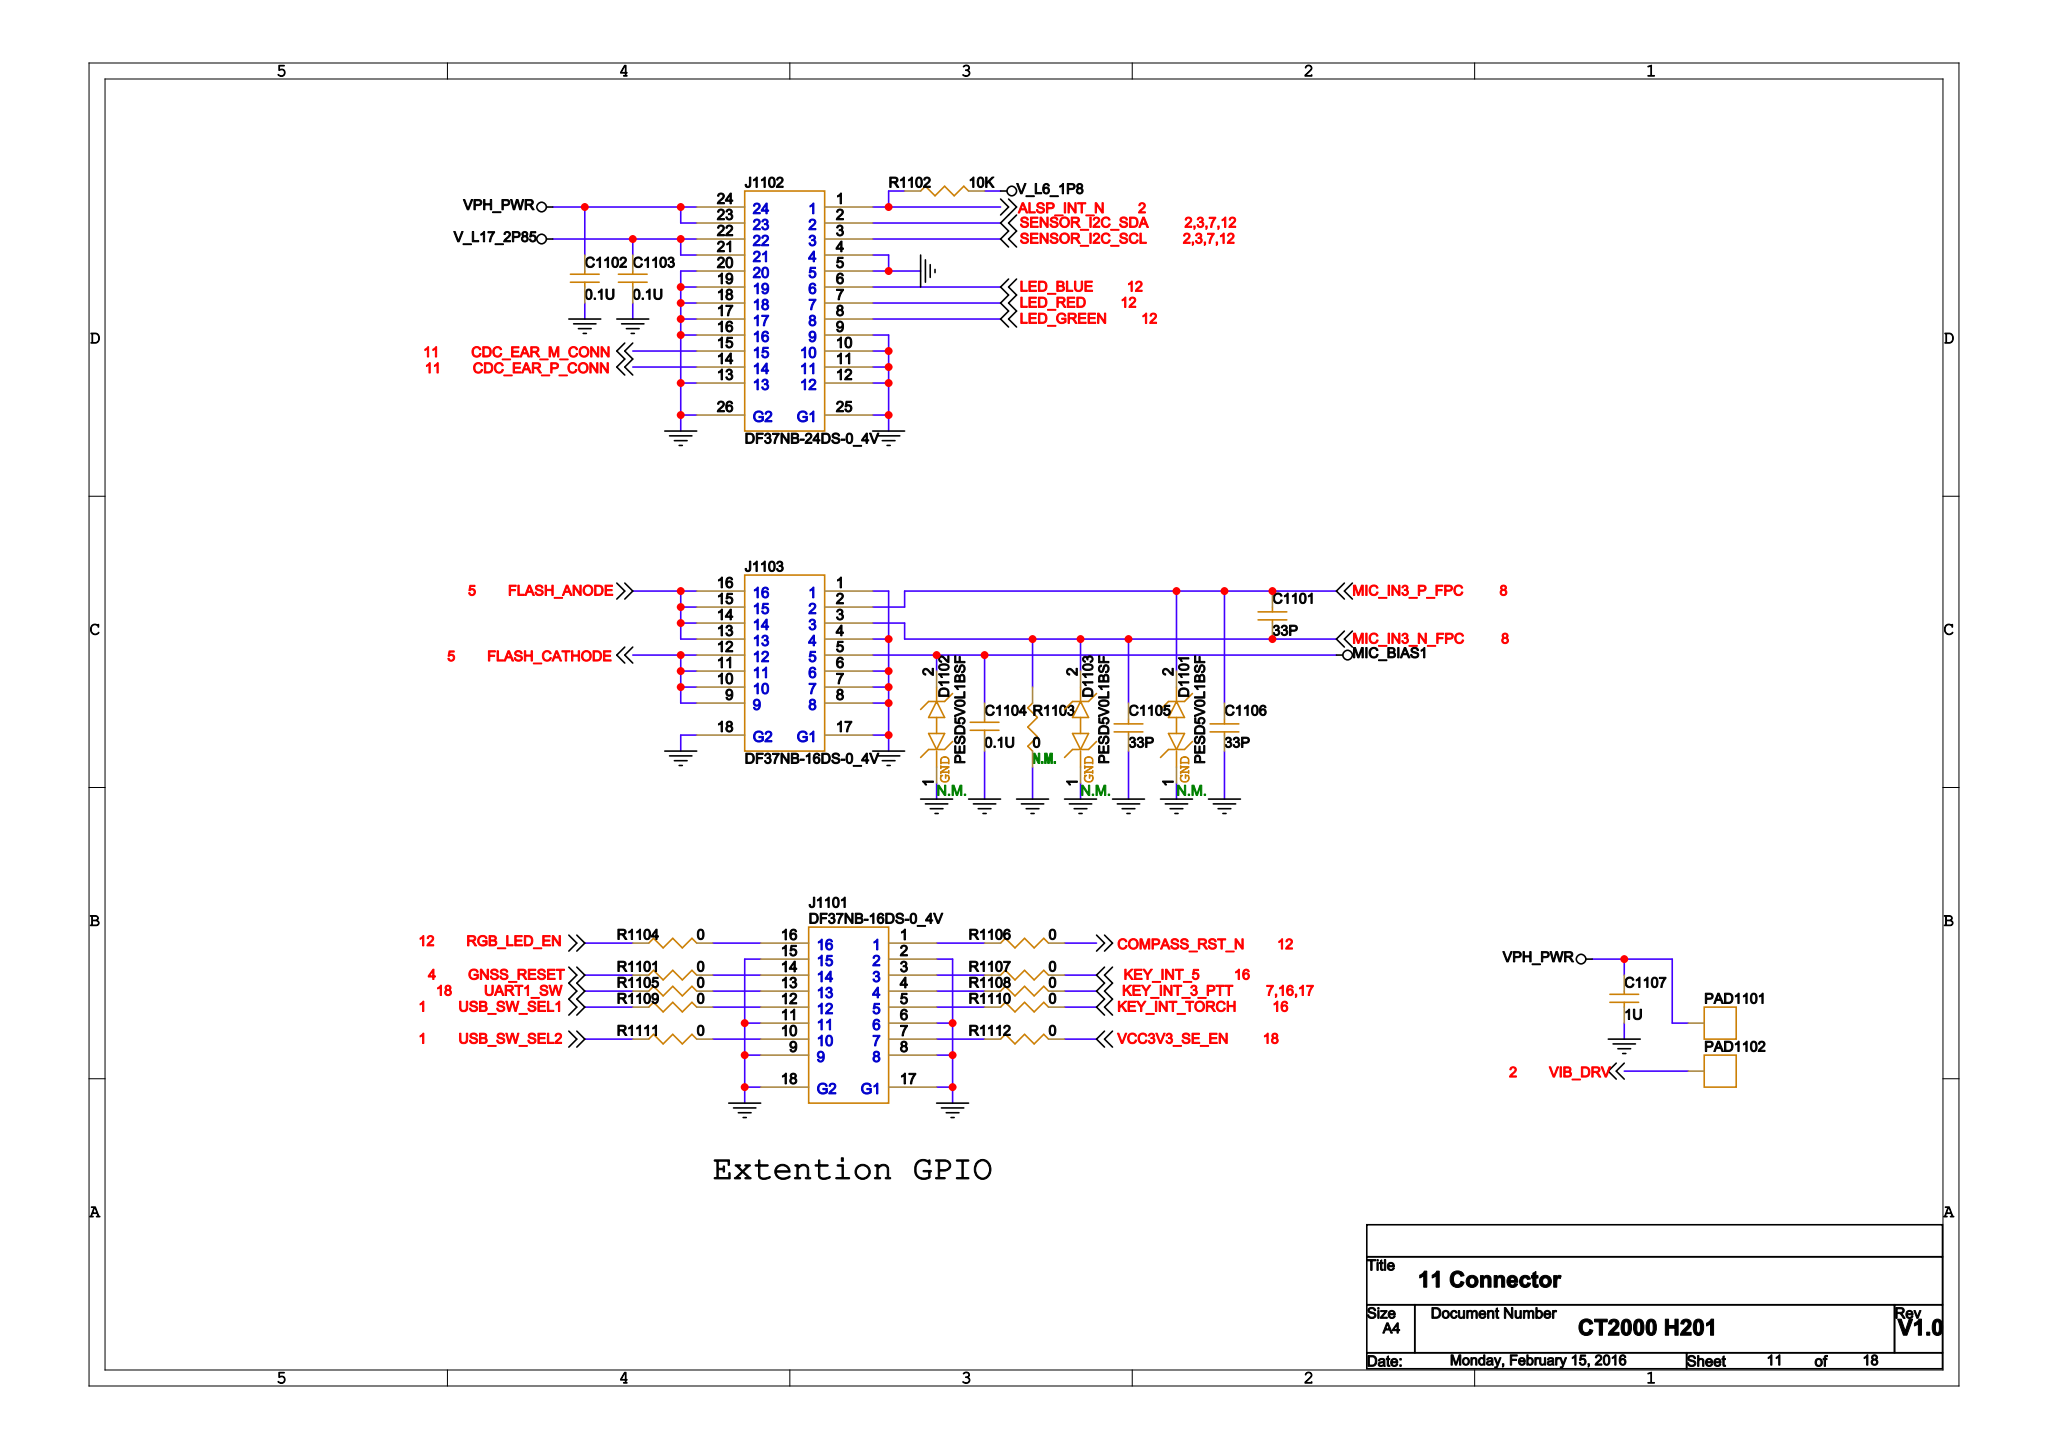Circuit board | Cadence Allegro | 573 parts | 376 nets | one sheet of the schematic
Parts on this sheet (reference | value | footprint):
C1101 | 33P | C0402
C1102 | 0.1U | C0402
C1103 | 0.1U | C0402
C1104 | 0.1U | C0402
C1105 | 33P | C0402
C1106 | 33P | C0402
C1107 | 1U | C0402
D1101 | PESD5V0L1BSF | DSN0603-2
D1102 | PESD5V0L1BSF | DSN0603-2
D1103 | PESD5V0L1BSF | DSN0603-2
J1101 | DF37NB-16DS-0_4V | BTB_DF37NB-16DS-0_4V_CW
J1102 | DF37NB-24DS-0_4V | BTB_DF37NB-24DS-0_4V_CW
J1103 | DF37NB-16DS-0_4V | BTB_DF37NB-16DS-0_4V_CW
PAD1101 | PAD_R1P2X2P2 | PAD_R1P5X2P7
PAD1102 | PAD_R1P2X2P2 | PAD_R1P5X2P7
R1101 | 0 | R0402
R1102 | 10K | R0402
R1103 | 0 | R0402
R1104 | 0 | R0402
R1105 | 0 | R0402
R1106 | 0 | R0402
R1107 | 0 | R0402
R1108 | 0 | R0402
R1109 | 0 | R0402
R1110 | 0 | R0402
R1111 | 0 | R0402
R1112 | 0 | R0402
Nets of these parts (net: part-pin ...):
GND: C1102-2 C1103-2 C1104-2 C1105-1 C1106-1 C1107-2 D1101-1 D1102-1 D1103-1 J1101-2 J1101-6 J1101-8 J1101-9 J1101-11 J1101-15 J1101-17 J1101-18 J1103-1 J1103-4 J1103-6 J1103-7 J1103-8 J1103-17 J1103-18 R1103-2 J1102-4 J1102-5 J1102-9 J1102-10 J1102-11 J1102-12 J1102-13 J1102-16 J1102-17 J1102-18 J1102-19 J1102-20 J1102-25 J1102-26
KEY_INT_3_PTT: R1108-2
KEY_INT_5: R1107-2
N52450270: J1101-1 R1106-1
N52817768: J1101-10 R1111-2
N52817747: J1101-12 R1109-2
N52817726: J1101-13 R1105-2
N52816759: J1101-14 R1101-2
N52816756: J1101-16 R1104-2
N52450276: J1101-3 R1107-1
N52450274: J1101-4 R1108-1
N52450359: J1101-5 R1110-1
N52450379: J1101-7 R1112-1
FLASH_CATHODE: J1103-9 J1103-10 J1103-11 J1103-12
FLASH_ANODE: J1103-13 J1103-14 J1103-15 J1103-16
MIC_IN3_P_FPC: C1101-2 C1106-2 D1101-2 J1103-2
MIC_IN3_N_FPC: C1101-1 C1105-2 D1103-2 J1103-3 R1103-1
MIC_BIAS1: C1104-1 D1102-2 J1103-5
ALSP_INT_N: R1102-1 J1102-1
CDC_EAR_P_CONN: J1102-14
CDC_EAR_M_CONN: J1102-15
SENSOR_I2C_SDA: J1102-2
V_L17_2P85: C1103-1 J1102-21 J1102-22
VPH_PWR: C1102-1 C1107-1 PAD1101-1 J1102-23 J1102-24
SENSOR_I2C_SCL: J1102-3
LED_BLUE: J1102-6
LED_RED: J1102-7
LED_GREEN: J1102-8
KEY_INT_TORCH: R1110-2
VIB_DRV: PAD1102-1
V_L6_1P8: R1102-2
VCC3V3_SE_EN: R1112-2
UART1_SW: R1105-1
USB_SW_SEL1: R1109-1
USB_SW_SEL2: R1111-1
COMPASS_RST_N: R1106-2
RGB_LED_EN: R1104-1
GNSS_RESET: R1101-1